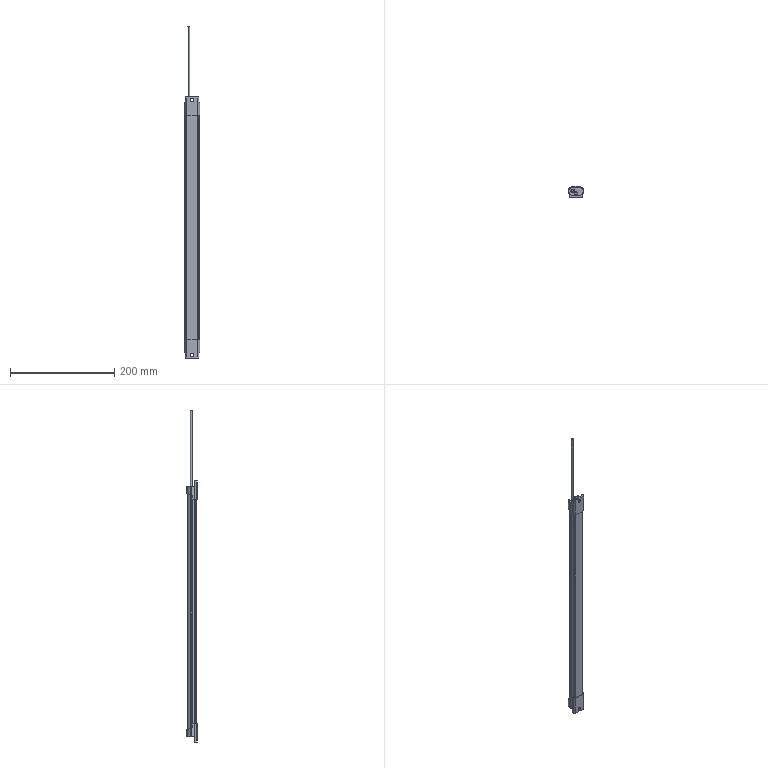Part | STEP file | 1 solid | 184 faces | box 30.32 x 21 x 636 mm | volume 212983 mm3 | cylinder 109 | plane 65 | torus 10 | commonest cylinder face diameters 4 x22 2 x9 14.8 x8 5 x6 12.02 x6 0.98 x4